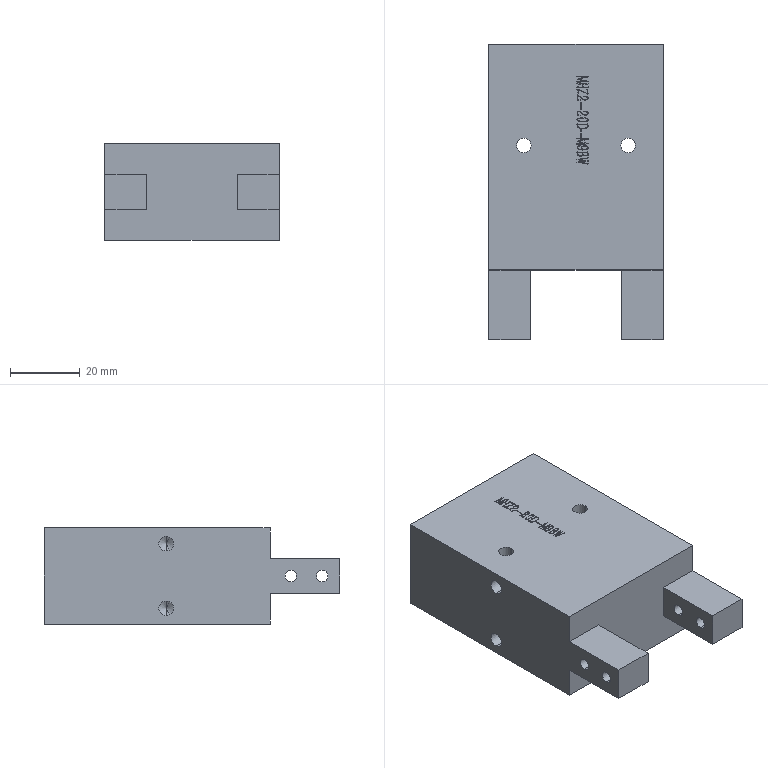Part | 1 solid | 300 faces | box 50 x 84.8 x 27.6 mm | volume 92760 mm3 | plane 177 | spline 103 | cylinder 16 | cone 4 | commonest cylinder face diameters 3.3 x8 4.2 x8